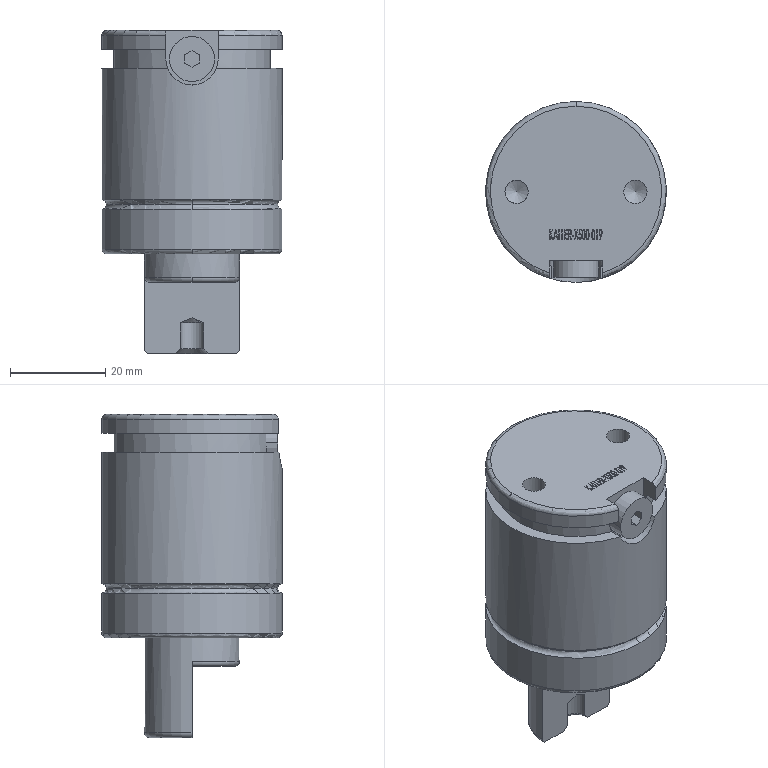Part | STEP file | 1_id1266_x_t | 1 solid | 180 faces | box 38 x 38 x 68 mm | volume 55593 mm3 | plane 130 | other 20 | torus 12 | cylinder 12 | cone 6 | commonest cylinder face diameters 4.9 x4 38 x3 9.5 x2 11 x1 20 x1 33 x1